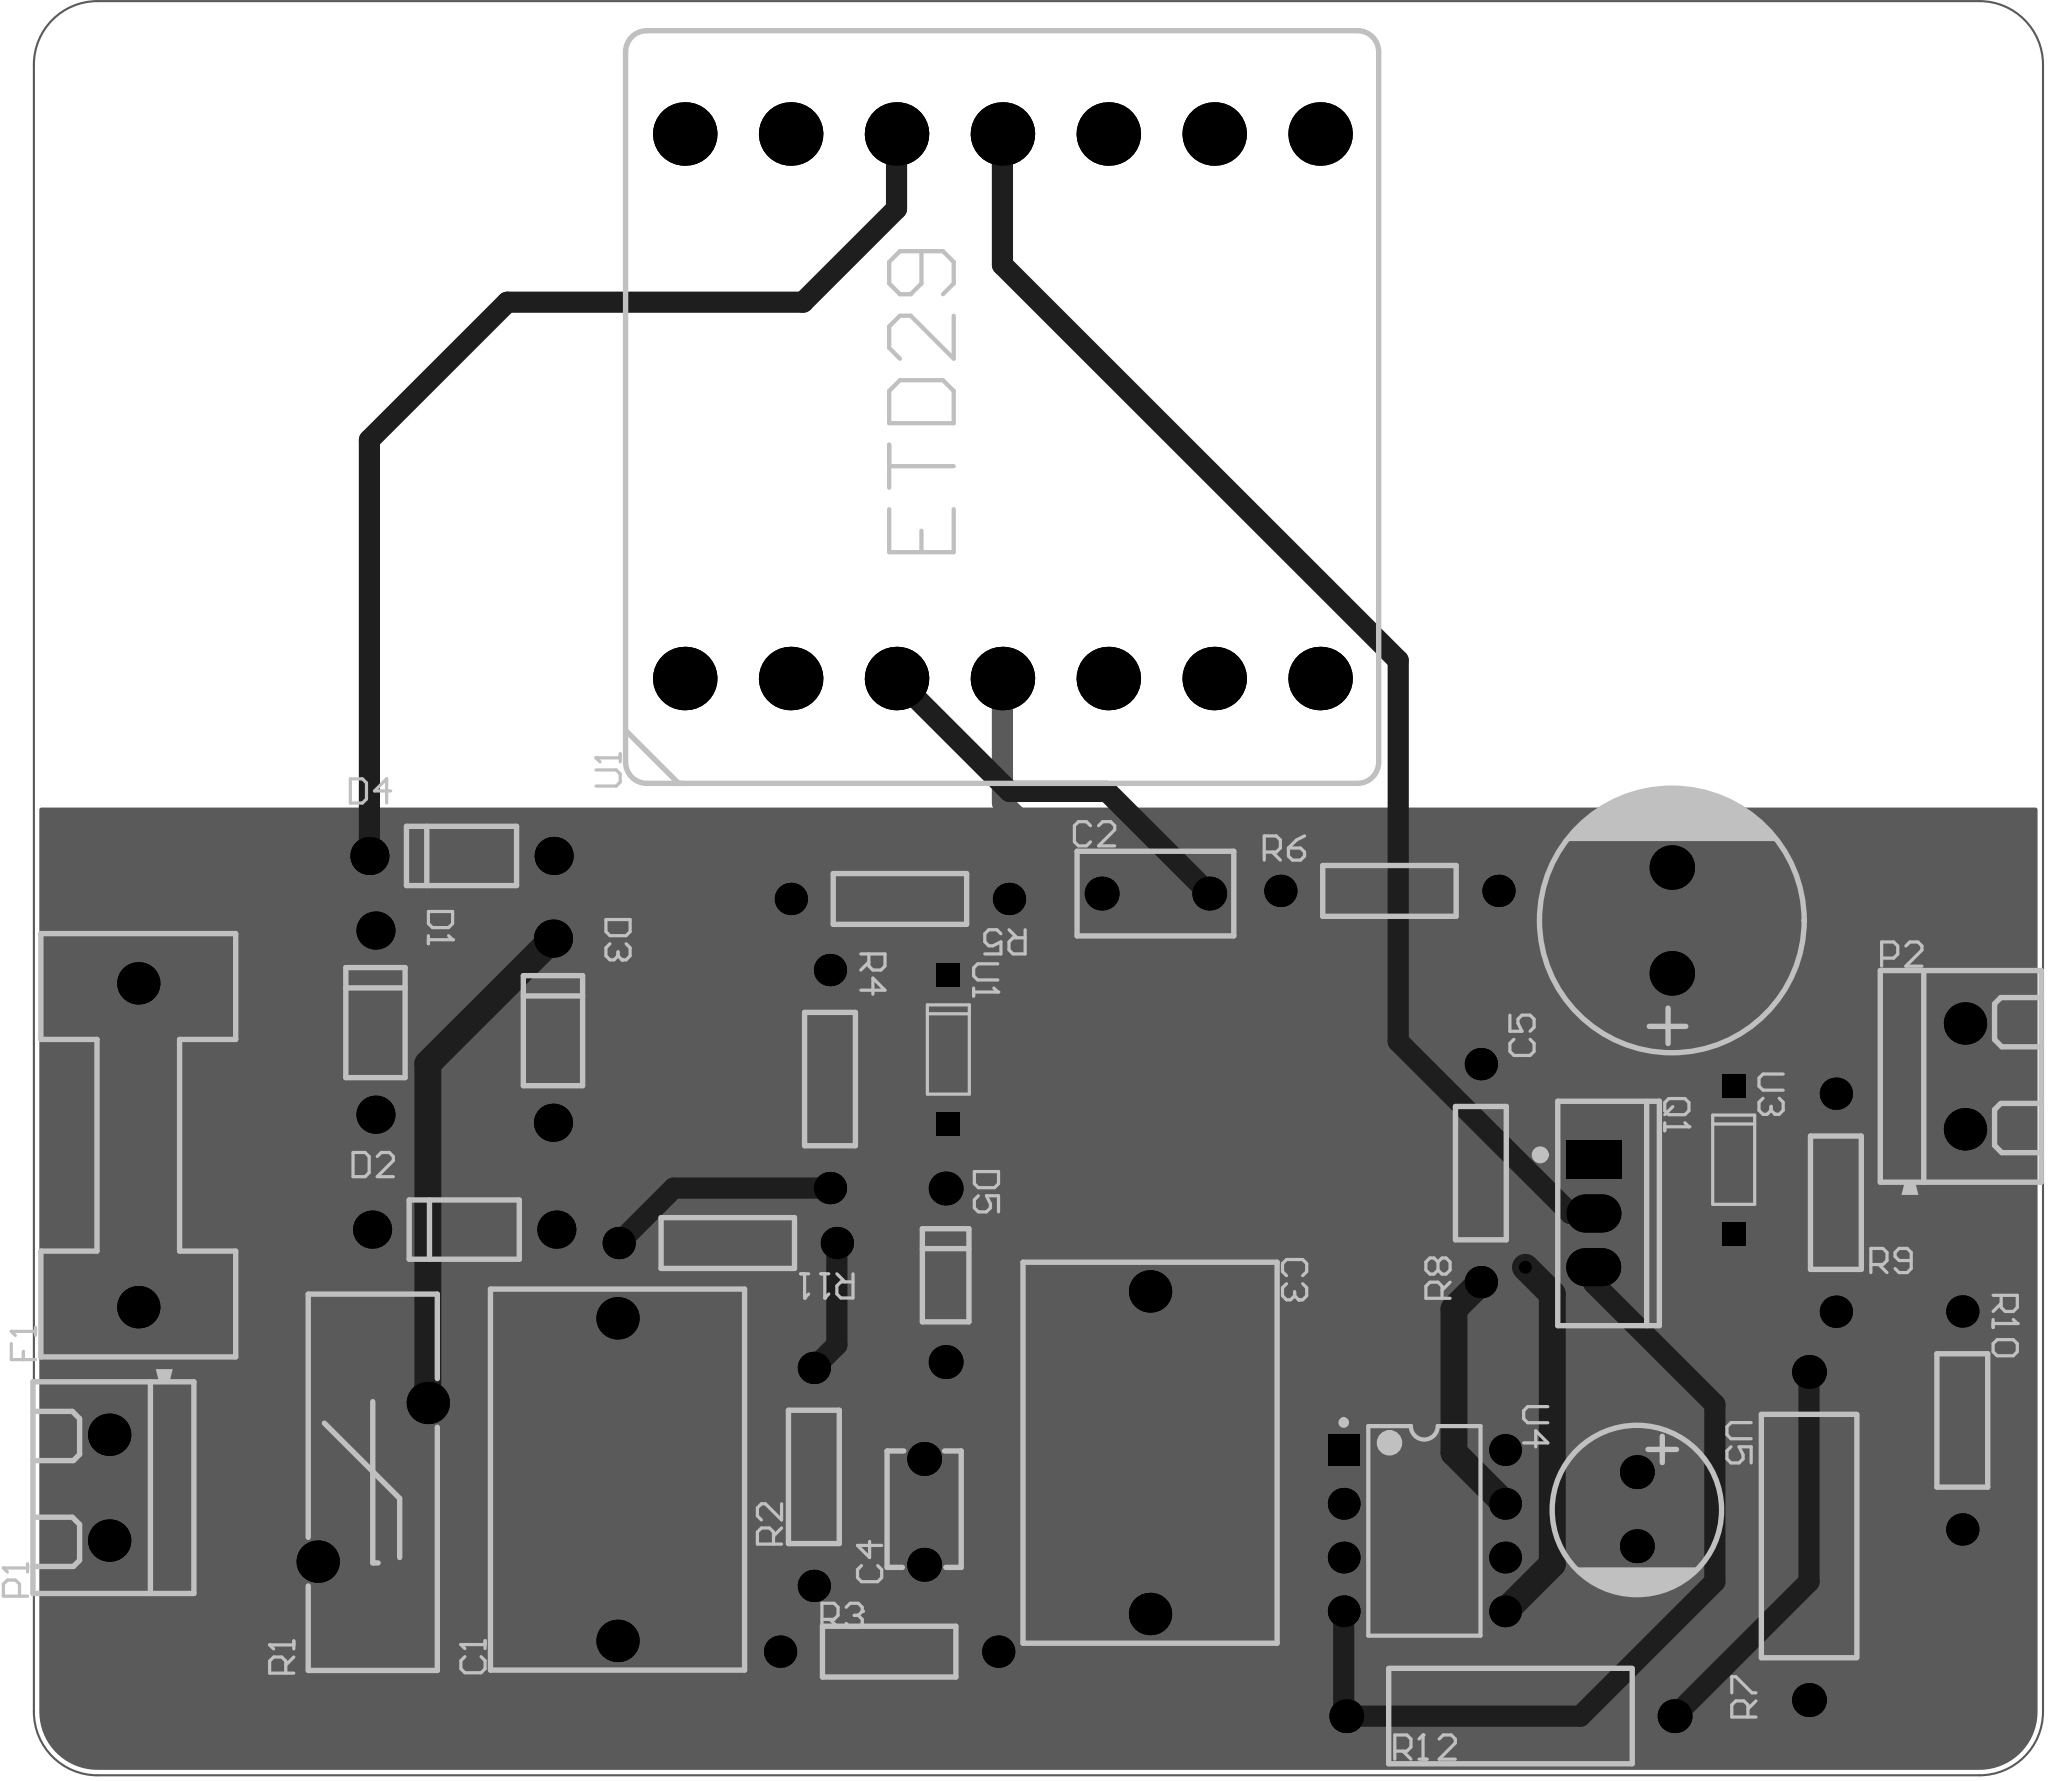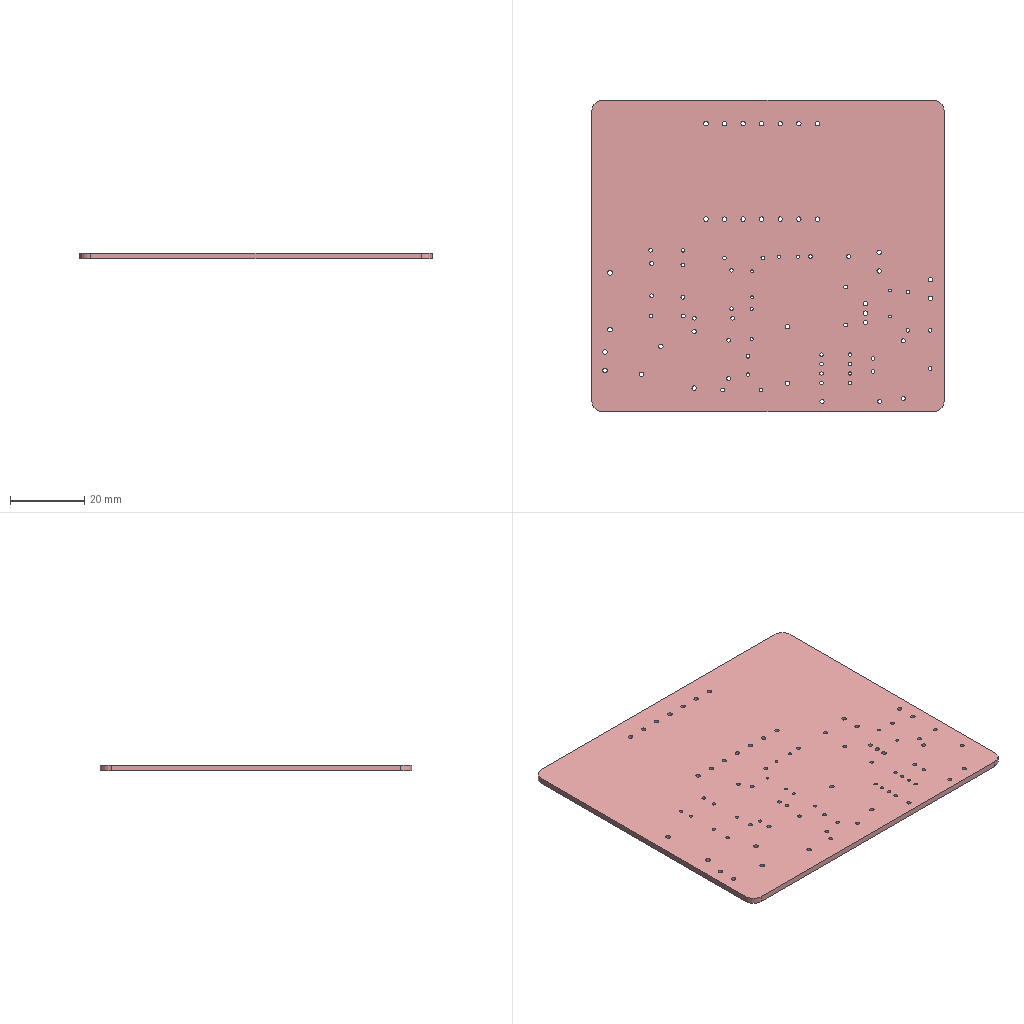Circuit board layout | Altium Designer | box 94.9 x 83.8 x 1.6 mm
Layer stack:
# Altium Designer layer stack of  (unit mm; dielectric type: 0 none, 1 core, 2 prepreg, 3 surface material)
index,name,kind,layer,copper_thickness_mm,dielectric_type,dielectric_thickness_mm,dielectric_material,dielectric_constant
0,Top Paste Mask Layer,other,,,,,,
1,Top Silkscreen Layer,other,,,,,,
2,Top Solder Mask Layer,dielectric,,,3,0.01,,3.3
3,Top Layer,copper,Top Layer,0.035,,,,
4,Dielectric1,dielectric,,,3,1.51,FR4,4.5
5,Bottom Layer,copper,Bottom Layer,0.035,,,,
6,Bottom Solder Mask Layer,dielectric,,,3,0.01,,3.3
7,Bottom Silkscreen Layer,other,,,,,,
8,Bottom Paste Mask Layer,other,,,,,,
# drill layer pairs: low layer,high layer
drill_pair,Top Layer,Bottom Layer
Part placement:
Designator,Comment,Layer,Footprint,Center-X(mm),Center-Y(mm),Rotation
C1,1uF,TopLayer,CAP-TH_L18.0-W12.0-P15.00-D1.2,106.045,90.932,90
C2,12nF,TopLayer,CAP-TH_L7.3-W4.0-P5.00-D0.5,131.445,118.618,0
C3,1uF,TopLayer,CAP-TH_L18.0-W12.0-P15.00-D1.2,131.191,92.202,270
C4,10nF,TopLayer,CAP-TH_L5.5-W3.5-P5.00-D1.2,120.523,89.408,90
C5,47uF,TopLayer,CAP-TH_BD12.5-P5.00-D0.6-FD,155.829,117.348,90
D1,,TopLayer,DO_1N4007,94.615,112.522,270
D2,,TopLayer,DO_1N4007,98.806,102.743,0
D3,,TopLayer,DO_1N4007,102.997,112.141,270
D4,,TopLayer,DO_1N4007,98.679,120.396,0
D5,1N5248B,TopLayer,DO-35_BD2.0-L4.2-P8.20-D0.5-RD,121.539,100.584,270
F1,5*20 fuse holder BF013,TopLayer,FUSE-TH_BF013,83.416,106.728,90
P1,KF301-2P terminal block,TopLayer,CONN-TH_XY301V-A-5.0-2P,82.042,90.551,90
P2,KF301-2P terminal block,TopLayer,CONN-TH_XY301V-A-5.0-2P,169.672,109.982,270
Q1,STP8NK80Z,TopLayer,TO-220-3_L10.0-W4.5-P2.54-L,152.146,103.505,270
R1,WTR15D050MC3BW,TopLayer,RES-TH_L17.5-W6.0-P7.50-D0.8-S5.20,94.488,90.805,90
R2,620K,TopLayer,Res_1/4W,115.316,91.059,90
R3,10KΩ,TopLayer,Res_1/4W,118.872,82.804,0
R4,240kΩ,TopLayer,Res_1/4W,116.078,109.855,270
R5,100Ω,TopLayer,Res_1/4W,119.38,118.364,180
R6,68kΩ,TopLayer,Res_1/4W,142.494,118.745,0
R7,0.22Ω,TopLayer,Res_1W,162.306,88.265,90
R8,10Ω,TopLayer,Res_1/4W,146.812,105.41,90
R9,998kΩ,TopLayer,Res_1/4W,163.576,104.013,270
R10,6.34kΩ,TopLayer,Res_1/4W,169.545,93.726,270
U1,1N4150TR,TopLayer,DO-35_BD1.8-L4.1-P7.00-D0.5-RD,121.666,111.252,270
U3,1N4150TR,TopLayer,DO-35_BD1.8-L4.1-P7.00-D0.5-RD,158.75,106.045,270
U4,L6561,TopLayer,DIP-8_L9.8-W6.6-P2.54-LS7.6-BL,144.145,88.519,270
U5,22UF400V,TopLayer,CAP-TH_BD8.0-P3.50-D0.6-FD,154.178,89.535,270
R11,620K,TopLayer,Res_1/4W,111.252,102.108,180
R12,0.22Ω,TopLayer,Res_1W,148.209,79.756,180
U1,,TopLayer,ETD29_ÎÔÊ½_14½Å·â×°,124.22,141.642,90
Pad and via stacks:
# Altium Designer via and pad stacks of  (unit mm). Each distinct definition once, with the count of objects using it.
# via: kind,start_layer,end_layer,hole_mm,diameter_mm,mode(0 simple;1 top-mid-bottom;2 full stack),diameter_per_layer,count,example_net
# pad: kind,layer,hole_mm,hole_type(0 round;1 square;2 slot),plating,top_size,top_shape(1 round;2 rect;3 octagon;9 rounded rect),mid_size,bottom_size,mode,footprint,size_per_layer,count,example
pad,Multi-Layer,1.2,0,plated,2x2,1,2x2,2x2,0,CAP-TH_L18.0-W12.0-P15.00-D1.2,,4,C1.1
pad,Multi-Layer,0.8,0,plated,1.6x1.6,1,1.6x1.6,1.6x1.6,0,CAP-TH_L7.3-W4.0-P5.00-D0.5,,2,C2.1
pad,Multi-Layer,1,0,plated,1.6x1.6,1,1.6x1.6,1.6x1.6,0,CAP-TH_L5.5-W3.5-P5.00-D1.2,,2,C4.1
pad,Multi-Layer,1.2,0,plated,2.1x2.1,1,2.1x2.1,2.1x2.1,0,CAP-TH_BD12.5-P5.00-D0.6-FD,,2,C5.1
pad,Multi-Layer,1,0,plated,1.8x1.8,1,1.8x1.8,1.8x1.8,0,DO_1N4007,,8,D1.1
pad,Multi-Layer,0.8,0,plated,1.6x1.6,1,1.6x1.6,1.6x1.6,0,DO-35_BD2.0-L4.2-P8.20-D0.5-RD,,2,D5.2
pad,Multi-Layer,1.3,0,plated,2x2,1,2x2,2x2,0,FUSE-TH_BF013,,2,F1.1
pad,Multi-Layer,1.2,0,plated,2x2,1,2x2,2x2,0,CONN-TH_XY301V-A-5.0-2P,,4,P1.1
pad,Multi-Layer,1.2,0,plated,1.8x2.6,1,1.8x2.6,1.8x2.6,0,TO-220-3_L10.0-W4.5-P2.54-L,,2,Q1.2
pad,Multi-Layer,1.2,0,plated,1.8x2.6,2,1.8x2.6,1.8x2.6,0,TO-220-3_L10.0-W4.5-P2.54-L,,1,Q1.1
pad,Multi-Layer,1.2,0,plated,2x2,1,2x2,2x2,0,RES-TH_L17.5-W6.0-P7.50-D0.8-S5.20,,2,R1.1
pad,Multi-Layer,1,0,plated,1.524x1.524,1,1.524x1.524,1.524x1.524,0,Res_1/4W,,18,R2.1
pad,Multi-Layer,1.1,0,plated,1.6x1.6,1,1.6x1.6,1.6x1.6,0,Res_1W,,4,R7.1
pad,Multi-Layer,0.73,0,plated,1.095x1.095,2,1.095x1.095,1.095x1.095,0,DO-35_BD1.8-L4.1-P7.00-D0.5-RD,,4,U1.1
pad,Multi-Layer,0.9,0,plated,1.5x1.5,2,1.5x1.5,1.5x1.5,0,DIP-8_L9.8-W6.6-P2.54-LS7.6-BL,,1,U4.1
pad,Multi-Layer,0.9,0,plated,1.5x1.5,1,1.5x1.5,1.5x1.5,0,DIP-8_L9.8-W6.6-P2.54-LS7.6-BL,,7,U4.2
pad,Multi-Layer,1,0,plated,1.6x1.6,1,1.6x1.6,1.6x1.6,0,CAP-TH_BD8.0-P3.50-D0.6-FD,,2,U5.2
pad,Multi-Layer,1.2,0,plated,3x3,1,3x3,3x3,0,ETD29 \u00CE\u00D4\u00CA\u00BD 14\u00BD\u00C5\u00B7\u00E2\u00D7\u00B0,,14,U1.1
via,Top Layer,Bottom Layer,0.3048,0.61,0,,1,$1N1946
Copper pours:
name,layer,net,type(0 solid;1 hatched;2 none)
Bottom Layer-GND,Bottom Layer,GND,0
Design rules, without the lines most boards share:
# Altium Designer design rules of  (exported by Altium Designer, unit mm)
# columns: name | kind | enabled | priority | scope1 | scope2 | descriptor | typed fields (field=value)
copperThickness1oz_2 | 2 | enabled | 2 | All | All | Width Constraint (Min=5mil) (Max=100mil) (Preferred=50mil) (All) |
viaSize | 11 | enabled | 1 | All | All | Routing Via (MinHoleWidth=11.811mil) (MaxHoleWidth=248.032mil) (PreferredHoleWidth=12.008mil) (MinWidth=19.685mil) (MaxWidth=393.701mil) (PreferedWidth=24.016mil) (All) | via_min_hole=0.3 via_max_hole=6.3 via_preferred_diameter=0.61 via_preferred_hole=0.305
solderMaskExpansion | 13 | enabled | 2 | All | All | Solder Mask Expansion (Expansion =2.008mil) (All) | expansion=0.051